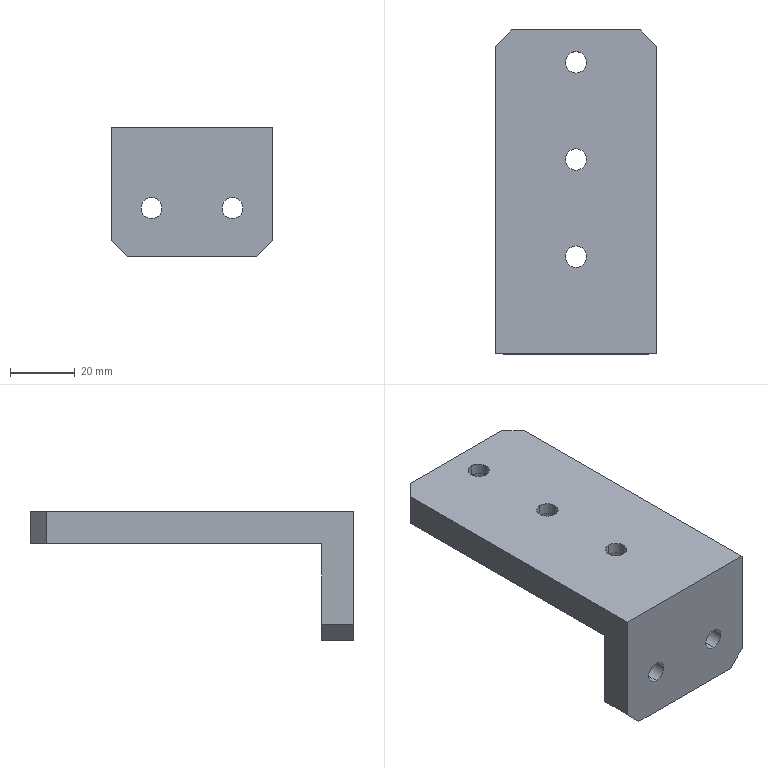Part | SolidWorks | features HoleWzd 2, Chamfer 1, ExtruThin 1 | 1 solid | 31 faces | box 50 x 100 x 40 mm | volume 61642 mm3 | cylinder 16 | plane 15 | commonest cylinder face diameters 6.6 x6 11 x6 6.5 x4
STEP:
#1=CARTESIAN_POINT('',(0.,84.5,-3.6));
#2=VERTEX_POINT('',#1);
#3=CARTESIAN_POINT('',(0.,95.5,-3.6));
#4=VERTEX_POINT('',#3);
#5=CARTESIAN_POINT('',(0.,90.,-3.6));
#6=DIRECTION('',(0.,0.,-1.));
#7=DIRECTION('',(0.,1.,0.));
#8=AXIS2_PLACEMENT_3D('',#5,#6,#7);
#9=CIRCLE('',#8,5.5);
#10=EDGE_CURVE('',#2,#4,#9,.T.);
#11=ORIENTED_EDGE('',*,*,#10,.F.);
#12=CARTESIAN_POINT('',(0.,84.5,-10.));
#13=VERTEX_POINT('',#12);
#14=CARTESIAN_POINT('',(0.,84.5,-10.));
#15=DIRECTION('',(0.,0.,-1.));
#16=VECTOR('',#15,1000.);
#17=LINE('',#14,#16);
#18=EDGE_CURVE('',#2,#13,#17,.T.);
#19=ORIENTED_EDGE('',*,*,#18,.T.);
#20=CARTESIAN_POINT('',(0.,95.5,-10.));
#21=VERTEX_POINT('',#20);
#22=CARTESIAN_POINT('',(0.,90.,-10.));
#23=DIRECTION('',(0.,0.,-1.));
#24=DIRECTION('',(0.,1.,0.));
#25=AXIS2_PLACEMENT_3D('',#22,#23,#24);
#26=CIRCLE('',#25,5.5);
#27=EDGE_CURVE('',#13,#21,#26,.T.);
#28=ORIENTED_EDGE('',*,*,#27,.T.);
#29=CARTESIAN_POINT('',(0.,95.5,-10.));
#30=DIRECTION('',(0.,0.,-1.));
#31=VECTOR('',#30,1000.);
#32=LINE('',#29,#31);
#33=EDGE_CURVE('',#4,#21,#32,.T.);
#34=ORIENTED_EDGE('',*,*,#33,.F.);
#35=EDGE_LOOP('',(#11,#19,#28,#34));
#36=FACE_OUTER_BOUND('',#35,.T.);
#37=CARTESIAN_POINT('',(0.,90.,-10.));
#38=DIRECTION('',(0.,0.,-1.));
#39=DIRECTION('',(0.,1.,0.));
#40=AXIS2_PLACEMENT_3D('',#37,#38,#39);
#41=CYLINDRICAL_SURFACE('',#40,5.5);
#42=ADVANCED_FACE('',(#36),#41,.F.);
#43=CARTESIAN_POINT('',(0.,86.7,0.));
#44=VERTEX_POINT('',#43);
#45=CARTESIAN_POINT('',(0.,93.3,0.));
#46=VERTEX_POINT('',#45);
#47=CARTESIAN_POINT('',(0.,90.,0.));
#48=DIRECTION('',(0.,0.,-1.));
#49=DIRECTION('',(0.,1.,0.));
#50=AXIS2_PLACEMENT_3D('',#47,#48,#49);
#51=CIRCLE('',#50,3.3);
#52=EDGE_CURVE('',#44,#46,#51,.T.);
#53=ORIENTED_EDGE('',*,*,#52,.F.);
#54=CARTESIAN_POINT('',(0.,86.7,-3.6));
#55=VERTEX_POINT('',#54);
#56=CARTESIAN_POINT('',(0.,86.7,-10.));
#57=DIRECTION('',(0.,0.,-1.));
#58=VECTOR('',#57,1000.);
#59=LINE('',#56,#58);
#60=EDGE_CURVE('',#44,#55,#59,.T.);
#61=ORIENTED_EDGE('',*,*,#60,.T.);
#62=CARTESIAN_POINT('',(0.,93.3,-3.6));
#63=VERTEX_POINT('',#62);
#64=CARTESIAN_POINT('',(0.,90.,-3.6));
#65=DIRECTION('',(0.,0.,-1.));
#66=DIRECTION('',(0.,1.,0.));
#67=AXIS2_PLACEMENT_3D('',#64,#65,#66);
#68=CIRCLE('',#67,3.3);
#69=EDGE_CURVE('',#55,#63,#68,.T.);
#70=ORIENTED_EDGE('',*,*,#69,.T.);
#71=CARTESIAN_POINT('',(0.,93.3,-10.));
#72=DIRECTION('',(0.,0.,-1.));
#73=VECTOR('',#72,1000.);
#74=LINE('',#71,#73);
#75=EDGE_CURVE('',#46,#63,#74,.T.);
#76=ORIENTED_EDGE('',*,*,#75,.F.);
#77=EDGE_LOOP('',(#53,#61,#70,#76));
#78=FACE_OUTER_BOUND('',#77,.T.);
#79=CARTESIAN_POINT('',(0.,90.,-10.));
#80=DIRECTION('',(0.,0.,-1.));
#81=DIRECTION('',(0.,1.,0.));
#82=AXIS2_PLACEMENT_3D('',#79,#80,#81);
#83=CYLINDRICAL_SURFACE('',#82,3.3);
#84=ADVANCED_FACE('',(#78),#83,.F.);
#85=CARTESIAN_POINT('',(0.,54.5,-3.6));
#86=VERTEX_POINT('',#85);
#87=CARTESIAN_POINT('',(0.,65.5,-3.6));
#88=VERTEX_POINT('',#87);
#89=CARTESIAN_POINT('',(0.,60.,-3.6));
#90=DIRECTION('',(0.,0.,-1.));
#91=DIRECTION('',(0.,1.,0.));
#92=AXIS2_PLACEMENT_3D('',#89,#90,#91);
#93=CIRCLE('',#92,5.5);
#94=EDGE_CURVE('',#86,#88,#93,.T.);
#95=ORIENTED_EDGE('',*,*,#94,.F.);
#96=CARTESIAN_POINT('',(0.,54.5,-10.));
#97=VERTEX_POINT('',#96);
#98=CARTESIAN_POINT('',(0.,54.5,-10.));
#99=DIRECTION('',(0.,0.,-1.));
#100=VECTOR('',#99,1000.);
#101=LINE('',#98,#100);
#102=EDGE_CURVE('',#86,#97,#101,.T.);
#103=ORIENTED_EDGE('',*,*,#102,.T.);
#104=CARTESIAN_POINT('',(0.,65.5,-10.));
#105=VERTEX_POINT('',#104);
#106=CARTESIAN_POINT('',(0.,60.,-10.));
#107=DIRECTION('',(0.,0.,-1.));
#108=DIRECTION('',(0.,1.,0.));
#109=AXIS2_PLACEMENT_3D('',#106,#107,#108);
#110=CIRCLE('',#109,5.5);
#111=EDGE_CURVE('',#97,#105,#110,.T.);
#112=ORIENTED_EDGE('',*,*,#111,.T.);
#113=CARTESIAN_POINT('',(0.,65.5,-10.));
#114=DIRECTION('',(0.,0.,-1.));
#115=VECTOR('',#114,1000.);
#116=LINE('',#113,#115);
#117=EDGE_CURVE('',#88,#105,#116,.T.);
#118=ORIENTED_EDGE('',*,*,#117,.F.);
#119=EDGE_LOOP('',(#95,#103,#112,#118));
#120=FACE_OUTER_BOUND('',#119,.T.);
#121=CARTESIAN_POINT('',(0.,60.,-10.));
#122=DIRECTION('',(0.,0.,-1.));
#123=DIRECTION('',(0.,1.,0.));
#124=AXIS2_PLACEMENT_3D('',#121,#122,#123);
#125=CYLINDRICAL_SURFACE('',#124,5.5);
#126=ADVANCED_FACE('',(#120),#125,.F.);
#127=CARTESIAN_POINT('',(0.,56.7,0.));
#128=VERTEX_POINT('',#127);
#129=CARTESIAN_POINT('',(0.,63.3,0.));
#130=VERTEX_POINT('',#129);
#131=CARTESIAN_POINT('',(0.,60.,0.));
#132=DIRECTION('',(0.,0.,-1.));
#133=DIRECTION('',(0.,1.,0.));
#134=AXIS2_PLACEMENT_3D('',#131,#132,#133);
#135=CIRCLE('',#134,3.3);
#136=EDGE_CURVE('',#128,#130,#135,.T.);
#137=ORIENTED_EDGE('',*,*,#136,.F.);
#138=CARTESIAN_POINT('',(0.,56.7,-3.6));
#139=VERTEX_POINT('',#138);
#140=CARTESIAN_POINT('',(0.,56.7,-10.));
#141=DIRECTION('',(0.,0.,-1.));
#142=VECTOR('',#141,1000.);
#143=LINE('',#140,#142);
#144=EDGE_CURVE('',#128,#139,#143,.T.);
#145=ORIENTED_EDGE('',*,*,#144,.T.);
#146=CARTESIAN_POINT('',(0.,63.3,-3.6));
#147=VERTEX_POINT('',#146);
#148=CARTESIAN_POINT('',(0.,60.,-3.6));
#149=DIRECTION('',(0.,0.,-1.));
#150=DIRECTION('',(0.,1.,0.));
#151=AXIS2_PLACEMENT_3D('',#148,#149,#150);
#152=CIRCLE('',#151,3.3);
#153=EDGE_CURVE('',#139,#147,#152,.T.);
#154=ORIENTED_EDGE('',*,*,#153,.T.);
#155=CARTESIAN_POINT('',(0.,63.3,-10.));
#156=DIRECTION('',(0.,0.,-1.));
#157=VECTOR('',#156,1000.);
#158=LINE('',#155,#157);
#159=EDGE_CURVE('',#130,#147,#158,.T.);
#160=ORIENTED_EDGE('',*,*,#159,.F.);
#161=EDGE_LOOP('',(#137,#145,#154,#160));
#162=FACE_OUTER_BOUND('',#161,.T.);
#163=CARTESIAN_POINT('',(0.,60.,-10.));
#164=DIRECTION('',(0.,0.,-1.));
#165=DIRECTION('',(0.,1.,0.));
#166=AXIS2_PLACEMENT_3D('',#163,#164,#165);
#167=CYLINDRICAL_SURFACE('',#166,3.3);
#168=ADVANCED_FACE('',(#162),#167,.F.);
#169=CARTESIAN_POINT('',(0.,24.5,-3.6));
#170=VERTEX_POINT('',#169);
#171=CARTESIAN_POINT('',(0.,35.5,-3.6));
#172=VERTEX_POINT('',#171);
#173=CARTESIAN_POINT('',(0.,30.,-3.6));
#174=DIRECTION('',(0.,0.,-1.));
#175=DIRECTION('',(0.,1.,0.));
#176=AXIS2_PLACEMENT_3D('',#173,#174,#175);
#177=CIRCLE('',#176,5.5);
#178=EDGE_CURVE('',#170,#172,#177,.T.);
#179=ORIENTED_EDGE('',*,*,#178,.F.);
#180=CARTESIAN_POINT('',(0.,24.5,-10.));
#181=VERTEX_POINT('',#180);
#182=CARTESIAN_POINT('',(0.,24.5,-10.));
#183=DIRECTION('',(0.,0.,-1.));
#184=VECTOR('',#183,1000.);
#185=LINE('',#182,#184);
#186=EDGE_CURVE('',#170,#181,#185,.T.);
#187=ORIENTED_EDGE('',*,*,#186,.T.);
#188=CARTESIAN_POINT('',(0.,35.5,-10.));
#189=VERTEX_POINT('',#188);
#190=CARTESIAN_POINT('',(0.,30.,-10.));
#191=DIRECTION('',(0.,0.,-1.));
#192=DIRECTION('',(0.,1.,0.));
#193=AXIS2_PLACEMENT_3D('',#190,#191,#192);
#194=CIRCLE('',#193,5.5);
#195=EDGE_CURVE('',#181,#189,#194,.T.);
#196=ORIENTED_EDGE('',*,*,#195,.T.);
#197=CARTESIAN_POINT('',(0.,35.5,-10.));
#198=DIRECTION('',(0.,0.,-1.));
#199=VECTOR('',#198,1000.);
#200=LINE('',#197,#199);
#201=EDGE_CURVE('',#172,#189,#200,.T.);
#202=ORIENTED_EDGE('',*,*,#201,.F.);
#203=EDGE_LOOP('',(#179,#187,#196,#202));
#204=FACE_OUTER_BOUND('',#203,.T.);
#205=CARTESIAN_POINT('',(0.,30.,-10.));
#206=DIRECTION('',(0.,0.,-1.));
#207=DIRECTION('',(0.,1.,0.));
#208=AXIS2_PLACEMENT_3D('',#205,#206,#207);
#209=CYLINDRICAL_SURFACE('',#208,5.5);
#210=ADVANCED_FACE('',(#204),#209,.F.);
#211=CARTESIAN_POINT('',(0.,26.7,0.));
#212=VERTEX_POINT('',#211);
#213=CARTESIAN_POINT('',(0.,33.3,0.));
#214=VERTEX_POINT('',#213);
#215=CARTESIAN_POINT('',(0.,30.,0.));
#216=DIRECTION('',(0.,0.,-1.));
#217=DIRECTION('',(0.,1.,0.));
#218=AXIS2_PLACEMENT_3D('',#215,#216,#217);
#219=CIRCLE('',#218,3.3);
#220=EDGE_CURVE('',#212,#214,#219,.T.);
#221=ORIENTED_EDGE('',*,*,#220,.F.);
#222=CARTESIAN_POINT('',(0.,26.7,-3.6));
#223=VERTEX_POINT('',#222);
#224=CARTESIAN_POINT('',(0.,26.7,-10.));
#225=DIRECTION('',(0.,0.,-1.));
#226=VECTOR('',#225,1000.);
#227=LINE('',#224,#226);
#228=EDGE_CURVE('',#212,#223,#227,.T.);
#229=ORIENTED_EDGE('',*,*,#228,.T.);
#230=CARTESIAN_POINT('',(0.,33.3,-3.6));
#231=VERTEX_POINT('',#230);
#232=CARTESIAN_POINT('',(0.,30.,-3.6));
#233=DIRECTION('',(0.,0.,-1.));
#234=DIRECTION('',(0.,1.,0.));
#235=AXIS2_PLACEMENT_3D('',#232,#233,#234);
#236=CIRCLE('',#235,3.3);
#237=EDGE_CURVE('',#223,#231,#236,.T.);
#238=ORIENTED_EDGE('',*,*,#237,.T.);
#239=CARTESIAN_POINT('',(0.,33.3,-10.));
#240=DIRECTION('',(0.,0.,-1.));
#241=VECTOR('',#240,1000.);
#242=LINE('',#239,#241);
#243=EDGE_CURVE('',#214,#231,#242,.T.);
#244=ORIENTED_EDGE('',*,*,#243,.F.);
#245=EDGE_LOOP('',(#221,#229,#238,#244));
#246=FACE_OUTER_BOUND('',#245,.T.);
#247=CARTESIAN_POINT('',(0.,30.,-10.));
#248=DIRECTION('',(0.,0.,-1.));
#249=DIRECTION('',(0.,1.,0.));
#250=AXIS2_PLACEMENT_3D('',#247,#248,#249);
#251=CYLINDRICAL_SURFACE('',#250,3.3);
#252=ADVANCED_FACE('',(#246),#251,.F.);
#253=CARTESIAN_POINT('',(-12.5,0.,-28.25));
#254=VERTEX_POINT('',#253);
#255=CARTESIAN_POINT('',(-12.5,0.,-21.75));
#256=VERTEX_POINT('',#255);
#257=CARTESIAN_POINT('',(-12.5,0.,-25.));
#258=DIRECTION('',(0.,1.,0.));
#259=DIRECTION('',(0.,0.,1.));
#260=AXIS2_PLACEMENT_3D('',#257,#258,#259);
#261=CIRCLE('',#260,3.25);
#262=EDGE_CURVE('',#254,#256,#261,.T.);
#263=ORIENTED_EDGE('',*,*,#262,.F.);
#264=CARTESIAN_POINT('',(-12.5,10.,-28.25));
#265=VERTEX_POINT('',#264);
#266=CARTESIAN_POINT('',(-12.5,10.,-28.25));
#267=DIRECTION('',(0.,1.,0.));
#268=VECTOR('',#267,1000.);
#269=LINE('',#266,#268);
#270=EDGE_CURVE('',#254,#265,#269,.T.);
#271=ORIENTED_EDGE('',*,*,#270,.T.);
#272=CARTESIAN_POINT('',(-12.5,10.,-21.75));
#273=VERTEX_POINT('',#272);
#274=CARTESIAN_POINT('',(-12.5,10.,-25.));
#275=DIRECTION('',(0.,1.,0.));
#276=DIRECTION('',(0.,0.,1.));
#277=AXIS2_PLACEMENT_3D('',#274,#275,#276);
#278=CIRCLE('',#277,3.25);
#279=EDGE_CURVE('',#265,#273,#278,.T.);
#280=ORIENTED_EDGE('',*,*,#279,.T.);
#281=CARTESIAN_POINT('',(-12.5,10.,-21.75));
#282=DIRECTION('',(0.,1.,0.));
#283=VECTOR('',#282,1000.);
#284=LINE('',#281,#283);
#285=EDGE_CURVE('',#256,#273,#284,.T.);
#286=ORIENTED_EDGE('',*,*,#285,.F.);
#287=EDGE_LOOP('',(#263,#271,#280,#286));
#288=FACE_OUTER_BOUND('',#287,.T.);
#289=CARTESIAN_POINT('',(-12.5,10.,-25.));
#290=DIRECTION('',(0.,1.,0.));
#291=DIRECTION('',(0.,0.,1.));
#292=AXIS2_PLACEMENT_3D('',#289,#290,#291);
#293=CYLINDRICAL_SURFACE('',#292,3.25);
#294=ADVANCED_FACE('',(#288),#293,.F.);
#295=CARTESIAN_POINT('',(12.5,0.,-28.25));
#296=VERTEX_POINT('',#295);
#297=CARTESIAN_POINT('',(12.5,0.,-21.75));
#298=VERTEX_POINT('',#297);
#299=CARTESIAN_POINT('',(12.5,0.,-25.));
#300=DIRECTION('',(0.,1.,0.));
#301=DIRECTION('',(0.,0.,1.));
#302=AXIS2_PLACEMENT_3D('',#299,#300,#301);
#303=CIRCLE('',#302,3.25);
#304=EDGE_CURVE('',#296,#298,#303,.T.);
#305=ORIENTED_EDGE('',*,*,#304,.F.);
#306=CARTESIAN_POINT('',(12.5,10.,-28.25));
#307=VERTEX_POINT('',#306);
#308=CARTESIAN_POINT('',(12.5,10.,-28.25));
#309=DIRECTION('',(0.,1.,0.));
#310=VECTOR('',#309,1000.);
#311=LINE('',#308,#310);
#312=EDGE_CURVE('',#296,#307,#311,.T.);
#313=ORIENTED_EDGE('',*,*,#312,.T.);
#314=CARTESIAN_POINT('',(12.5,10.,-21.75));
#315=VERTEX_POINT('',#314);
#316=CARTESIAN_POINT('',(12.5,10.,-25.));
#317=DIRECTION('',(0.,1.,0.));
#318=DIRECTION('',(0.,0.,1.));
#319=AXIS2_PLACEMENT_3D('',#316,#317,#318);
#320=CIRCLE('',#319,3.25);
#321=EDGE_CURVE('',#307,#315,#320,.T.);
#322=ORIENTED_EDGE('',*,*,#321,.T.);
#323=CARTESIAN_POINT('',(12.5,10.,-21.75));
#324=DIRECTION('',(0.,1.,0.));
#325=VECTOR('',#324,1000.);
#326=LINE('',#323,#325);
#327=EDGE_CURVE('',#298,#315,#326,.T.);
#328=ORIENTED_EDGE('',*,*,#327,.F.);
#329=EDGE_LOOP('',(#305,#313,#322,#328));
#330=FACE_OUTER_BOUND('',#329,.T.);
#331=CARTESIAN_POINT('',(12.5,10.,-25.));
#332=DIRECTION('',(0.,1.,0.));
#333=DIRECTION('',(0.,0.,1.));
#334=AXIS2_PLACEMENT_3D('',#331,#332,#333);
#335=CYLINDRICAL_SURFACE('',#334,3.25);
#336=ADVANCED_FACE('',(#330),#335,.F.);
#337=CARTESIAN_POINT('',(-12.5,0.,-25.));
#338=DIRECTION('',(0.,1.,0.));
#339=DIRECTION('',(0.,0.,1.));
#340=AXIS2_PLACEMENT_3D('',#337,#338,#339);
#341=CIRCLE('',#340,3.25);
#342=EDGE_CURVE('',#256,#254,#341,.T.);
#343=ORIENTED_EDGE('',*,*,#342,.T.);
#344=ORIENTED_EDGE('',*,*,#262,.T.);
#345=EDGE_LOOP('',(#343,#344));
#346=FACE_BOUND('',#345,.T.);
#347=CARTESIAN_POINT('',(12.5,0.,-25.));
#348=DIRECTION('',(0.,1.,0.));
#349=DIRECTION('',(0.,0.,1.));
#350=AXIS2_PLACEMENT_3D('',#347,#348,#349);
#351=CIRCLE('',#350,3.25);
#352=EDGE_CURVE('',#298,#296,#351,.T.);
#353=ORIENTED_EDGE('',*,*,#352,.T.);
#354=ORIENTED_EDGE('',*,*,#304,.T.);
#355=EDGE_LOOP('',(#353,#354));
#356=FACE_BOUND('',#355,.T.);
#357=CARTESIAN_POINT('',(-25.,0.,0.));
#358=VERTEX_POINT('',#357);
#359=CARTESIAN_POINT('',(-25.,0.,-35.));
#360=VERTEX_POINT('',#359);
#361=CARTESIAN_POINT('',(-25.,0.,0.));
#362=DIRECTION('',(0.,0.,-1.));
#363=VECTOR('',#362,1000.);
#364=LINE('',#361,#363);
#365=EDGE_CURVE('',#358,#360,#364,.T.);
#366=ORIENTED_EDGE('',*,*,#365,.T.);
#367=CARTESIAN_POINT('',(-20.,0.,-40.));
#368=VERTEX_POINT('',#367);
#369=CARTESIAN_POINT('',(-25.,0.,-35.));
#370=DIRECTION('',(0.7071,0.,-0.7071));
#371=VECTOR('',#370,1000.);
#372=LINE('',#369,#371);
#373=EDGE_CURVE('',#360,#368,#372,.T.);
#374=ORIENTED_EDGE('',*,*,#373,.T.);
#375=CARTESIAN_POINT('',(20.,0.,-40.));
#376=VERTEX_POINT('',#375);
#377=CARTESIAN_POINT('',(25.,0.,-40.));
#378=DIRECTION('',(-1.,0.,0.));
#379=VECTOR('',#378,1000.);
#380=LINE('',#377,#379);
#381=EDGE_CURVE('',#376,#368,#380,.T.);
#382=ORIENTED_EDGE('',*,*,#381,.F.);
#383=CARTESIAN_POINT('',(25.,0.,-35.));
#384=VERTEX_POINT('',#383);
#385=CARTESIAN_POINT('',(20.,0.,-40.));
#386=DIRECTION('',(0.7071,0.,0.7071));
#387=VECTOR('',#386,1000.);
#388=LINE('',#385,#387);
#389=EDGE_CURVE('',#376,#384,#388,.T.);
#390=ORIENTED_EDGE('',*,*,#389,.T.);
#391=CARTESIAN_POINT('',(25.,0.,0.));
#392=VERTEX_POINT('',#391);
#393=CARTESIAN_POINT('',(25.,0.,0.));
#394=DIRECTION('',(0.,0.,-1.));
#395=VECTOR('',#394,1000.);
#396=LINE('',#393,#395);
#397=EDGE_CURVE('',#392,#384,#396,.T.);
#398=ORIENTED_EDGE('',*,*,#397,.F.);
#399=CARTESIAN_POINT('',(25.,0.,0.));
#400=DIRECTION('',(-1.,0.,0.));
#401=VECTOR('',#400,1000.);
#402=LINE('',#399,#401);
#403=EDGE_CURVE('',#392,#358,#402,.T.);
#404=ORIENTED_EDGE('',*,*,#403,.T.);
#405=EDGE_LOOP('',(#366,#374,#382,#390,#398,#404));
#406=FACE_OUTER_BOUND('',#405,.T.);
#407=CARTESIAN_POINT('',(25.,0.,0.));
#408=DIRECTION('',(0.,1.,0.));
#409=DIRECTION('',(0.,0.,1.));
#410=AXIS2_PLACEMENT_3D('',#407,#408,#409);
#411=PLANE('',#410);
#412=ADVANCED_FACE('',(#346,#356,#406),#411,.F.);
#413=ORIENTED_EDGE('',*,*,#381,.T.);
#414=CARTESIAN_POINT('',(-20.,10.,-40.));
#415=VERTEX_POINT('',#414);
#416=CARTESIAN_POINT('',(-20.,10.,-40.));
#417=DIRECTION('',(0.,1.,0.));
#418=VECTOR('',#417,1000.);
#419=LINE('',#416,#418);
#420=EDGE_CURVE('',#368,#415,#419,.T.);
#421=ORIENTED_EDGE('',*,*,#420,.T.);
#422=CARTESIAN_POINT('',(20.,10.,-40.));
#423=VERTEX_POINT('',#422);
#424=CARTESIAN_POINT('',(25.,10.,-40.));
#425=DIRECTION('',(-1.,0.,0.));
#426=VECTOR('',#425,1000.);
#427=LINE('',#424,#426);
#428=EDGE_CURVE('',#423,#415,#427,.T.);
#429=ORIENTED_EDGE('',*,*,#428,.F.);
#430=CARTESIAN_POINT('',(20.,0.,-40.));
#431=DIRECTION('',(0.,-1.,0.));
#432=VECTOR('',#431,1000.);
#433=LINE('',#430,#432);
#434=EDGE_CURVE('',#423,#376,#433,.T.);
#435=ORIENTED_EDGE('',*,*,#434,.T.);
#436=EDGE_LOOP('',(#413,#421,#429,#435));
#437=FACE_OUTER_BOUND('',#436,.T.);
#438=CARTESIAN_POINT('',(25.,10.,-40.));
#439=DIRECTION('',(0.,0.,-1.));
#440=DIRECTION('',(-1.,0.,0.));
#441=AXIS2_PLACEMENT_3D('',#438,#439,#440);
#442=PLANE('',#441);
#443=ADVANCED_FACE('',(#437),#442,.T.);
#444=CARTESIAN_POINT('',(-12.5,10.,-25.));
#445=DIRECTION('',(0.,1.,0.));
#446=DIRECTION('',(0.,0.,1.));
#447=AXIS2_PLACEMENT_3D('',#444,#445,#446);
#448=CIRCLE('',#447,3.25);
#449=EDGE_CURVE('',#273,#265,#448,.T.);
#450=ORIENTED_EDGE('',*,*,#449,.F.);
#451=ORIENTED_EDGE('',*,*,#279,.F.);
#452=EDGE_LOOP('',(#450,#451));
#453=FACE_BOUND('',#452,.T.);
#454=CARTESIAN_POINT('',(12.5,10.,-25.));
#455=DIRECTION('',(0.,1.,0.));
#456=DIRECTION('',(0.,0.,1.));
#457=AXIS2_PLACEMENT_3D('',#454,#455,#456);
#458=CIRCLE('',#457,3.25);
#459=EDGE_CURVE('',#315,#307,#458,.T.);
#460=ORIENTED_EDGE('',*,*,#459,.F.);
#461=ORIENTED_EDGE('',*,*,#321,.F.);
#462=EDGE_LOOP('',(#460,#461));
#463=FACE_BOUND('',#462,.T.);
#464=ORIENTED_EDGE('',*,*,#428,.T.);
#465=CARTESIAN_POINT('',(-25.,10.,-35.));
#466=VERTEX_POINT('',#465);
#467=CARTESIAN_POINT('',(-17.5,10.,-42.5));
#468=DIRECTION('',(-0.7071,0.,0.7071));
#469=VECTOR('',#468,1000.);
#470=LINE('',#467,#469);
#471=EDGE_CURVE('',#415,#466,#470,.T.);
#472=ORIENTED_EDGE('',*,*,#471,.T.);
#473=CARTESIAN_POINT('',(-25.,10.,-10.));
#474=VERTEX_POINT('',#473);
#475=CARTESIAN_POINT('',(-25.,10.,0.));
#476=DIRECTION('',(0.,0.,-1.));
#477=VECTOR('',#476,1000.);
#478=LINE('',#475,#477);
#479=EDGE_CURVE('',#474,#466,#478,.T.);
#480=ORIENTED_EDGE('',*,*,#479,.F.);
#481=CARTESIAN_POINT('',(25.,10.,-10.));
#482=VERTEX_POINT('',#481);
#483=CARTESIAN_POINT('',(25.,10.,-10.));
#484=DIRECTION('',(-1.,0.,0.));
#485=VECTOR('',#484,1000.);
#486=LINE('',#483,#485);
#487=EDGE_CURVE('',#482,#474,#486,.T.);
#488=ORIENTED_EDGE('',*,*,#487,.F.);
#489=CARTESIAN_POINT('',(25.,10.,-35.));
#490=VERTEX_POINT('',#489);
#491=CARTESIAN_POINT('',(25.,10.,0.));
#492=DIRECTION('',(0.,0.,-1.));
#493=VECTOR('',#492,1000.);
#494=LINE('',#491,#493);
#495=EDGE_CURVE('',#482,#490,#494,.T.);
#496=ORIENTED_EDGE('',*,*,#495,.T.);
#497=CARTESIAN_POINT('',(42.5,10.,-17.5));
#498=DIRECTION('',(-0.7071,0.,-0.7071));
#499=VECTOR('',#498,1000.);
#500=LINE('',#497,#499);
#501=EDGE_CURVE('',#490,#423,#500,.T.);
#502=ORIENTED_EDGE('',*,*,#501,.T.);
#503=EDGE_LOOP('',(#464,#472,#480,#488,#496,#502));
#504=FACE_OUTER_BOUND('',#503,.T.);
#505=CARTESIAN_POINT('',(25.,10.,0.));
#506=DIRECTION('',(0.,1.,0.));
#507=DIRECTION('',(0.,0.,1.));
#508=AXIS2_PLACEMENT_3D('',#505,#506,#507);
#509=PLANE('',#508);
#510=ADVANCED_FACE('',(#453,#463,#504),#509,.T.);
#511=CARTESIAN_POINT('',(0.,90.,-10.));
#512=DIRECTION('',(0.,0.,-1.));
#513=DIRECTION('',(0.,1.,0.));
#514=AXIS2_PLACEMENT_3D('',#511,#512,#513);
#515=CIRCLE('',#514,5.5);
#516=EDGE_CURVE('',#21,#13,#515,.T.);
#517=ORIENTED_EDGE('',*,*,#516,.F.);
#518=ORIENTED_EDGE('',*,*,#27,.F.);
#519=EDGE_LOOP('',(#517,#518));
#520=FACE_BOUND('',#519,.T.);
#521=CARTESIAN_POINT('',(0.,60.,-10.));
#522=DIRECTION('',(0.,0.,-1.));
#523=DIRECTION('',(0.,1.,0.));
#524=AXIS2_PLACEMENT_3D('',#521,#522,#523);
#525=CIRCLE('',#524,5.5);
#526=EDGE_CURVE('',#105,#97,#525,.T.);
#527=ORIENTED_EDGE('',*,*,#526,.F.);
#528=ORIENTED_EDGE('',*,*,#111,.F.);
#529=EDGE_LOOP('',(#527,#528));
#530=FACE_BOUND('',#529,.T.);
#531=CARTESIAN_POINT('',(0.,30.,-10.));
#532=DIRECTION('',(0.,0.,-1.));
#533=DIRECTION('',(0.,1.,0.));
#534=AXIS2_PLACEMENT_3D('',#531,#532,#533);
#535=CIRCLE('',#534,5.5);
#536=EDGE_CURVE('',#189,#181,#535,.T.);
#537=ORIENTED_EDGE('',*,*,#536,.F.);
#538=ORIENTED_EDGE('',*,*,#195,.F.);
#539=EDGE_LOOP('',(#537,#538));
#540=FACE_BOUND('',#539,.T.);
#541=CARTESIAN_POINT('',(-25.,95.,-10.));
#542=VERTEX_POINT('',#541);
#543=CARTESIAN_POINT('',(-25.,100.,-10.));
#544=DIRECTION('',(0.,-1.,0.));
#545=VECTOR('',#544,1000.);
#546=LINE('',#543,#545);
#547=EDGE_CURVE('',#542,#474,#546,.T.);
#548=ORIENTED_EDGE('',*,*,#547,.F.);
#549=CARTESIAN_POINT('',(-20.,100.,-10.));
#550=VERTEX_POINT('',#549);
#551=CARTESIAN_POINT('',(2.5,122.5,-10.));
#552=DIRECTION('',(0.7071,0.7071,0.));
#553=VECTOR('',#552,1000.);
#554=LINE('',#551,#553);
#555=EDGE_CURVE('',#542,#550,#554,.T.);
#556=ORIENTED_EDGE('',*,*,#555,.T.);
#557=CARTESIAN_POINT('',(20.,100.,-10.));
#558=VERTEX_POINT('',#557);
#559=CARTESIAN_POINT('',(25.,100.,-10.));
#560=DIRECTION('',(-1.,0.,0.));
#561=VECTOR('',#560,1000.);
#562=LINE('',#559,#561);
#563=EDGE_CURVE('',#558,#550,#562,.T.);
#564=ORIENTED_EDGE('',*,*,#563,.F.);
#565=CARTESIAN_POINT('',(25.,95.,-10.));
#566=VERTEX_POINT('',#565);
#567=CARTESIAN_POINT('',(22.5,97.5,-10.));
#568=DIRECTION('',(0.7071,-0.7071,0.));
#569=VECTOR('',#568,1000.);
#570=LINE('',#567,#569);
#571=EDGE_CURVE('',#558,#566,#570,.T.);
#572=ORIENTED_EDGE('',*,*,#571,.T.);
#573=CARTESIAN_POINT('',(25.,100.,-10.));
#574=DIRECTION('',(0.,-1.,0.));
#575=VECTOR('',#574,1000.);
#576=LINE('',#573,#575);
#577=EDGE_CURVE('',#566,#482,#576,.T.);
#578=ORIENTED_EDGE('',*,*,#577,.T.);
#579=ORIENTED_EDGE('',*,*,#487,.T.);
#580=EDGE_LOOP('',(#548,#556,#564,#572,#578,#579));
#581=FACE_OUTER_BOUND('',#580,.T.);
#582=CARTESIAN_POINT('',(25.,100.,-10.));
#583=DIRECTION('',(0.,0.,-1.));
#584=DIRECTION('',(0.,1.,0.));
#585=AXIS2_PLACEMENT_3D('',#582,#583,#584);
#586=PLANE('',#585);
#587=ADVANCED_FACE('',(#520,#530,#540,#581),#586,.T.);
#588=ORIENTED_EDGE('',*,*,#563,.T.);
#589=CARTESIAN_POINT('',(-20.,100.,0.));
#590=VERTEX_POINT('',#589);
#591=CARTESIAN_POINT('',(-20.,100.,0.));
#592=DIRECTION('',(0.,0.,1.));
#593=VECTOR('',#592,1000.);
#594=LINE('',#591,#593);
#595=EDGE_CURVE('',#550,#590,#594,.T.);
#596=ORIENTED_EDGE('',*,*,#595,.T.);
#597=CARTESIAN_POINT('',(20.,100.,0.));
#598=VERTEX_POINT('',#597);
#599=CARTESIAN_POINT('',(25.,100.,0.));
#600=DIRECTION('',(-1.,0.,0.));
#601=VECTOR('',#600,1000.);
#602=LINE('',#599,#601);
#603=EDGE_CURVE('',#598,#590,#602,.T.);
#604=ORIENTED_EDGE('',*,*,#603,.F.);
#605=CARTESIAN_POINT('',(20.,100.,-10.));
#606=DIRECTION('',(0.,0.,-1.));
#607=VECTOR('',#606,1000.);
#608=LINE('',#605,#607);
#609=EDGE_CURVE('',#598,#558,#608,.T.);
#610=ORIENTED_EDGE('',*,*,#609,.T.);
#611=EDGE_LOOP('',(#588,#596,#604,#610));
#612=FACE_OUTER_BOUND('',#611,.T.);
#613=CARTESIAN_POINT('',(25.,100.,0.));
#614=DIRECTION('',(0.,1.,0.));
#615=DIRECTION('',(0.,0.,1.));
#616=AXIS2_PLACEMENT_3D('',#613,#614,#615);
#617=PLANE('',#616);
#618=ADVANCED_FACE('',(#612),#617,.T.);
#619=CARTESIAN_POINT('',(0.,90.,0.));
#620=DIRECTION('',(0.,0.,-1.));
#621=DIRECTION('',(0.,1.,0.));
#622=AXIS2_PLACEMENT_3D('',#619,#620,#621);
#623=CIRCLE('',#622,3.3);
#624=EDGE_CURVE('',#46,#44,#623,.T.);
#625=ORIENTED_EDGE('',*,*,#624,.T.);
#626=ORIENTED_EDGE('',*,*,#52,.T.);
#627=EDGE_LOOP('',(#625,#626));
#628=FACE_BOUND('',#627,.T.);
#629=CARTESIAN_POINT('',(0.,60.,0.));
#630=DIRECTION('',(0.,0.,-1.));
#631=DIRECTION('',(0.,1.,0.));
#632=AXIS2_PLACEMENT_3D('',#629,#630,#631);
#633=CIRCLE('',#632,3.3);
#634=EDGE_CURVE('',#130,#128,#633,.T.);
#635=ORIENTED_EDGE('',*,*,#634,.T.);
#636=ORIENTED_EDGE('',*,*,#136,.T.);
#637=EDGE_LOOP('',(#635,#636));
#638=FACE_BOUND('',#637,.T.);
#639=CARTESIAN_POINT('',(0.,30.,0.));
#640=DIRECTION('',(0.,0.,-1.));
#641=DIRECTION('',(0.,1.,0.));
#642=AXIS2_PLACEMENT_3D('',#639,#640,#641);
#643=CIRCLE('',#642,3.3);
#644=EDGE_CURVE('',#214,#212,#643,.T.);
#645=ORIENTED_EDGE('',*,*,#644,.T.);
#646=ORIENTED_EDGE('',*,*,#220,.T.);
#647=EDGE_LOOP('',(#645,#646));
#648=FACE_BOUND('',#647,.T.);
#649=ORIENTED_EDGE('',*,*,#603,.T.);
#650=CARTESIAN_POINT('',(-25.,95.,0.));
#651=VERTEX_POINT('',#650);
#652=CARTESIAN_POINT('',(-25.,95.,0.));
#653=DIRECTION('',(-0.7071,-0.7071,0.));
#654=VECTOR('',#653,1000.);
#655=LINE('',#652,#654);
#656=EDGE_CURVE('',#590,#651,#655,.T.);
#657=ORIENTED_EDGE('',*,*,#656,.T.);
#658=CARTESIAN_POINT('',(-25.,100.,0.));
#659=DIRECTION('',(0.,-1.,0.));
#660=VECTOR('',#659,1000.);
#661=LINE('',#658,#660);
#662=EDGE_CURVE('',#651,#358,#661,.T.);
#663=ORIENTED_EDGE('',*,*,#662,.T.);
#664=ORIENTED_EDGE('',*,*,#403,.F.);
#665=CARTESIAN_POINT('',(25.,95.,0.));
#666=VERTEX_POINT('',#665);
#667=CARTESIAN_POINT('',(25.,100.,0.));
#668=DIRECTION('',(0.,-1.,0.));
#669=VECTOR('',#668,1000.);
#670=LINE('',#667,#669);
#671=EDGE_CURVE('',#666,#392,#670,.T.);
#672=ORIENTED_EDGE('',*,*,#671,.F.);
#673=CARTESIAN_POINT('',(20.,100.,0.));
#674=DIRECTION('',(-0.7071,0.7071,0.));
#675=VECTOR('',#674,1000.);
#676=LINE('',#673,#675);
#677=EDGE_CURVE('',#666,#598,#676,.T.);
#678=ORIENTED_EDGE('',*,*,#677,.T.);
#679=EDGE_LOOP('',(#649,#657,#663,#664,#672,#678));
#680=FACE_OUTER_BOUND('',#679,.T.);
#681=CARTESIAN_POINT('',(25.,100.,0.));
#682=DIRECTION('',(0.,0.,-1.));
#683=DIRECTION('',(0.,1.,0.));
#684=AXIS2_PLACEMENT_3D('',#681,#682,#683);
#685=PLANE('',#684);
#686=ADVANCED_FACE('',(#628,#638,#648,#680),#685,.F.);
#687=ORIENTED_EDGE('',*,*,#397,.T.);
#688=CARTESIAN_POINT('',(25.,10.,-35.));
#689=DIRECTION('',(0.,1.,0.));
#690=VECTOR('',#689,1000.);
#691=LINE('',#688,#690);
#692=EDGE_CURVE('',#384,#490,#691,.T.);
#693=ORIENTED_EDGE('',*,*,#692,.T.);
#694=ORIENTED_EDGE('',*,*,#495,.F.);
#695=ORIENTED_EDGE('',*,*,#577,.F.);
#696=CARTESIAN_POINT('',(25.,95.,0.));
#697=DIRECTION('',(0.,0.,1.));
#698=VECTOR('',#697,1000.);
#699=LINE('',#696,#698);
#700=EDGE_CURVE('',#566,#666,#699,.T.);
#701=ORIENTED_EDGE('',*,*,#700,.T.);
#702=ORIENTED_EDGE('',*,*,#671,.T.);
#703=EDGE_LOOP('',(#687,#693,#694,#695,#701,#702));
#704=FACE_OUTER_BOUND('',#703,.T.);
#705=CARTESIAN_POINT('',(25.,0.,0.));
#706=DIRECTION('',(-1.,0.,0.));
#707=DIRECTION('',(0.,0.,1.));
#708=AXIS2_PLACEMENT_3D('',#705,#706,#707);
#709=PLANE('',#708);
#710=ADVANCED_FACE('',(#704),#709,.F.);
#711=ORIENTED_EDGE('',*,*,#479,.T.);
#712=CARTESIAN_POINT('',(-25.,0.,-35.));
#713=DIRECTION('',(0.,-1.,0.));
#714=VECTOR('',#713,1000.);
#715=LINE('',#712,#714);
#716=EDGE_CURVE('',#466,#360,#715,.T.);
#717=ORIENTED_EDGE('',*,*,#716,.T.);
#718=ORIENTED_EDGE('',*,*,#365,.F.);
#719=ORIENTED_EDGE('',*,*,#662,.F.);
#720=CARTESIAN_POINT('',(-25.,95.,0.));
#721=DIRECTION('',(0.,0.,-1.));
#722=VECTOR('',#721,1000.);
#723=LINE('',#720,#722);
#724=EDGE_CURVE('',#651,#542,#723,.T.);
#725=ORIENTED_EDGE('',*,*,#724,.T.);
#726=ORIENTED_EDGE('',*,*,#547,.T.);
#727=EDGE_LOOP('',(#711,#717,#718,#719,#725,#726));
#728=FACE_OUTER_BOUND('',#727,.T.);
#729=CARTESIAN_POINT('',(-25.,0.,0.));
#730=DIRECTION('',(-1.,0.,0.));
#731=DIRECTION('',(0.,0.,1.));
#732=AXIS2_PLACEMENT_3D('',#729,#730,#731);
#733=PLANE('',#732);
#734=ADVANCED_FACE('',(#728),#733,.T.);
#735=ORIENTED_EDGE('',*,*,#312,.F.);
#736=ORIENTED_EDGE('',*,*,#352,.F.);
#737=ORIENTED_EDGE('',*,*,#327,.T.);
#738=ORIENTED_EDGE('',*,*,#459,.T.);
#739=EDGE_LOOP('',(#735,#736,#737,#738));
#740=FACE_OUTER_BOUND('',#739,.T.);
#741=CARTESIAN_POINT('',(12.5,10.,-25.));
#742=DIRECTION('',(0.,1.,0.));
#743=DIRECTION('',(0.,0.,1.));
#744=AXIS2_PLACEMENT_3D('',#741,#742,#743);
#745=CYLINDRICAL_SURFACE('',#744,3.25);
#746=ADVANCED_FACE('',(#740),#745,.F.);
#747=ORIENTED_EDGE('',*,*,#270,.F.);
#748=ORIENTED_EDGE('',*,*,#342,.F.);
#749=ORIENTED_EDGE('',*,*,#285,.T.);
#750=ORIENTED_EDGE('',*,*,#449,.T.);
#751=EDGE_LOOP('',(#747,#748,#749,#750));
#752=FACE_OUTER_BOUND('',#751,.T.);
#753=CARTESIAN_POINT('',(-12.5,10.,-25.));
#754=DIRECTION('',(0.,1.,0.));
#755=DIRECTION('',(0.,0.,1.));
#756=AXIS2_PLACEMENT_3D('',#753,#754,#755);
#757=CYLINDRICAL_SURFACE('',#756,3.25);
#758=ADVANCED_FACE('',(#752),#757,.F.);
#759=ORIENTED_EDGE('',*,*,#228,.F.);
#760=ORIENTED_EDGE('',*,*,#644,.F.);
#761=ORIENTED_EDGE('',*,*,#243,.T.);
#762=CARTESIAN_POINT('',(0.,30.,-3.6));
#763=DIRECTION('',(0.,0.,-1.));
#764=DIRECTION('',(0.,1.,0.));
#765=AXIS2_PLACEMENT_3D('',#762,#763,#764);
#766=CIRCLE('',#765,3.3);
#767=EDGE_CURVE('',#231,#223,#766,.T.);
#768=ORIENTED_EDGE('',*,*,#767,.T.);
#769=EDGE_LOOP('',(#759,#760,#761,#768));
#770=FACE_OUTER_BOUND('',#769,.T.);
#771=CARTESIAN_POINT('',(0.,30.,-10.));
#772=DIRECTION('',(0.,0.,-1.));
#773=DIRECTION('',(0.,1.,0.));
#774=AXIS2_PLACEMENT_3D('',#771,#772,#773);
#775=CYLINDRICAL_SURFACE('',#774,3.3);
#776=ADVANCED_FACE('',(#770),#775,.F.);
#777=ORIENTED_EDGE('',*,*,#767,.F.);
#778=ORIENTED_EDGE('',*,*,#237,.F.);
#779=EDGE_LOOP('',(#777,#778));
#780=FACE_BOUND('',#779,.T.);
#781=CARTESIAN_POINT('',(0.,30.,-3.6));
#782=DIRECTION('',(0.,0.,-1.));
#783=DIRECTION('',(0.,1.,0.));
#784=AXIS2_PLACEMENT_3D('',#781,#782,#783);
#785=CIRCLE('',#784,5.5);
#786=EDGE_CURVE('',#172,#170,#785,.T.);
#787=ORIENTED_EDGE('',*,*,#786,.T.);
#788=ORIENTED_EDGE('',*,*,#178,.T.);
#789=EDGE_LOOP('',(#787,#788));
#790=FACE_OUTER_BOUND('',#789,.T.);
#791=CARTESIAN_POINT('',(3.3,30.,-3.6));
#792=DIRECTION('',(0.,0.,1.));
#793=DIRECTION('',(0.,-1.,0.));
#794=AXIS2_PLACEMENT_3D('',#791,#792,#793);
#795=PLANE('',#794);
#796=ADVANCED_FACE('',(#780,#790),#795,.F.);
#797=ORIENTED_EDGE('',*,*,#186,.F.);
#798=ORIENTED_EDGE('',*,*,#786,.F.);
#799=ORIENTED_EDGE('',*,*,#201,.T.);
#800=ORIENTED_EDGE('',*,*,#536,.T.);
#801=EDGE_LOOP('',(#797,#798,#799,#800));
#802=FACE_OUTER_BOUND('',#801,.T.);
#803=CARTESIAN_POINT('',(0.,30.,-10.));
#804=DIRECTION('',(0.,0.,-1.));
#805=DIRECTION('',(0.,1.,0.));
#806=AXIS2_PLACEMENT_3D('',#803,#804,#805);
#807=CYLINDRICAL_SURFACE('',#806,5.5);
#808=ADVANCED_FACE('',(#802),#807,.F.);
#809=ORIENTED_EDGE('',*,*,#144,.F.);
#810=ORIENTED_EDGE('',*,*,#634,.F.);
#811=ORIENTED_EDGE('',*,*,#159,.T.);
#812=CARTESIAN_POINT('',(0.,60.,-3.6));
#813=DIRECTION('',(0.,0.,-1.));
#814=DIRECTION('',(0.,1.,0.));
#815=AXIS2_PLACEMENT_3D('',#812,#813,#814);
#816=CIRCLE('',#815,3.3);
#817=EDGE_CURVE('',#147,#139,#816,.T.);
#818=ORIENTED_EDGE('',*,*,#817,.T.);
#819=EDGE_LOOP('',(#809,#810,#811,#818));
#820=FACE_OUTER_BOUND('',#819,.T.);
#821=CARTESIAN_POINT('',(0.,60.,-10.));
#822=DIRECTION('',(0.,0.,-1.));
#823=DIRECTION('',(0.,1.,0.));
#824=AXIS2_PLACEMENT_3D('',#821,#822,#823);
#825=CYLINDRICAL_SURFACE('',#824,3.3);
#826=ADVANCED_FACE('',(#820),#825,.F.);
#827=ORIENTED_EDGE('',*,*,#817,.F.);
#828=ORIENTED_EDGE('',*,*,#153,.F.);
#829=EDGE_LOOP('',(#827,#828));
#830=FACE_BOUND('',#829,.T.);
#831=CARTESIAN_POINT('',(0.,60.,-3.6));
#832=DIRECTION('',(0.,0.,-1.));
#833=DIRECTION('',(0.,1.,0.));
#834=AXIS2_PLACEMENT_3D('',#831,#832,#833);
#835=CIRCLE('',#834,5.5);
#836=EDGE_CURVE('',#88,#86,#835,.T.);
#837=ORIENTED_EDGE('',*,*,#836,.T.);
#838=ORIENTED_EDGE('',*,*,#94,.T.);
#839=EDGE_LOOP('',(#837,#838));
#840=FACE_OUTER_BOUND('',#839,.T.);
#841=CARTESIAN_POINT('',(3.3,60.,-3.6));
#842=DIRECTION('',(0.,0.,1.));
#843=DIRECTION('',(0.,-1.,0.));
#844=AXIS2_PLACEMENT_3D('',#841,#842,#843);
#845=PLANE('',#844);
#846=ADVANCED_FACE('',(#830,#840),#845,.F.);
#847=ORIENTED_EDGE('',*,*,#102,.F.);
#848=ORIENTED_EDGE('',*,*,#836,.F.);
#849=ORIENTED_EDGE('',*,*,#117,.T.);
#850=ORIENTED_EDGE('',*,*,#526,.T.);
#851=EDGE_LOOP('',(#847,#848,#849,#850));
#852=FACE_OUTER_BOUND('',#851,.T.);
#853=CARTESIAN_POINT('',(0.,60.,-10.));
#854=DIRECTION('',(0.,0.,-1.));
#855=DIRECTION('',(0.,1.,0.));
#856=AXIS2_PLACEMENT_3D('',#853,#854,#855);
#857=CYLINDRICAL_SURFACE('',#856,5.5);
#858=ADVANCED_FACE('',(#852),#857,.F.);
#859=ORIENTED_EDGE('',*,*,#60,.F.);
#860=ORIENTED_EDGE('',*,*,#624,.F.);
#861=ORIENTED_EDGE('',*,*,#75,.T.);
#862=CARTESIAN_POINT('',(0.,90.,-3.6));
#863=DIRECTION('',(0.,0.,-1.));
#864=DIRECTION('',(0.,1.,0.));
#865=AXIS2_PLACEMENT_3D('',#862,#863,#864);
#866=CIRCLE('',#865,3.3);
#867=EDGE_CURVE('',#63,#55,#866,.T.);
#868=ORIENTED_EDGE('',*,*,#867,.T.);
#869=EDGE_LOOP('',(#859,#860,#861,#868));
#870=FACE_OUTER_BOUND('',#869,.T.);
#871=CARTESIAN_POINT('',(0.,90.,-10.));
#872=DIRECTION('',(0.,0.,-1.));
#873=DIRECTION('',(0.,1.,0.));
#874=AXIS2_PLACEMENT_3D('',#871,#872,#873);
#875=CYLINDRICAL_SURFACE('',#874,3.3);
#876=ADVANCED_FACE('',(#870),#875,.F.);
#877=ORIENTED_EDGE('',*,*,#867,.F.);
#878=ORIENTED_EDGE('',*,*,#69,.F.);
#879=EDGE_LOOP('',(#877,#878));
#880=FACE_BOUND('',#879,.T.);
#881=CARTESIAN_POINT('',(0.,90.,-3.6));
#882=DIRECTION('',(0.,0.,-1.));
#883=DIRECTION('',(0.,1.,0.));
#884=AXIS2_PLACEMENT_3D('',#881,#882,#883);
#885=CIRCLE('',#884,5.5);
#886=EDGE_CURVE('',#4,#2,#885,.T.);
#887=ORIENTED_EDGE('',*,*,#886,.T.);
#888=ORIENTED_EDGE('',*,*,#10,.T.);
#889=EDGE_LOOP('',(#887,#888));
#890=FACE_OUTER_BOUND('',#889,.T.);
#891=CARTESIAN_POINT('',(3.3,90.,-3.6));
#892=DIRECTION('',(0.,0.,1.));
#893=DIRECTION('',(0.,-1.,0.));
#894=AXIS2_PLACEMENT_3D('',#891,#892,#893);
#895=PLANE('',#894);
#896=ADVANCED_FACE('',(#880,#890),#895,.F.);
#897=ORIENTED_EDGE('',*,*,#18,.F.);
#898=ORIENTED_EDGE('',*,*,#886,.F.);
#899=ORIENTED_EDGE('',*,*,#33,.T.);
#900=ORIENTED_EDGE('',*,*,#516,.T.);
#901=EDGE_LOOP('',(#897,#898,#899,#900));
#902=FACE_OUTER_BOUND('',#901,.T.);
#903=CARTESIAN_POINT('',(0.,90.,-10.));
#904=DIRECTION('',(0.,0.,-1.));
#905=DIRECTION('',(0.,1.,0.));
#906=AXIS2_PLACEMENT_3D('',#903,#904,#905);
#907=CYLINDRICAL_SURFACE('',#906,5.5);
#908=ADVANCED_FACE('',(#902),#907,.F.);
#909=ORIENTED_EDGE('',*,*,#471,.F.);
#910=ORIENTED_EDGE('',*,*,#420,.F.);
#911=ORIENTED_EDGE('',*,*,#373,.F.);
#912=ORIENTED_EDGE('',*,*,#716,.F.);
#913=EDGE_LOOP('',(#909,#910,#911,#912));
#914=FACE_OUTER_BOUND('',#913,.T.);
#915=CARTESIAN_POINT('',(-25.,0.,-35.));
#916=DIRECTION('',(0.7071,0.,0.7071));
#917=DIRECTION('',(0.,-1.,0.));
#918=AXIS2_PLACEMENT_3D('',#915,#916,#917);
#919=PLANE('',#918);
#920=ADVANCED_FACE('',(#914),#919,.F.);
#921=ORIENTED_EDGE('',*,*,#501,.F.);
#922=ORIENTED_EDGE('',*,*,#692,.F.);
#923=ORIENTED_EDGE('',*,*,#389,.F.);
#924=ORIENTED_EDGE('',*,*,#434,.F.);
#925=EDGE_LOOP('',(#921,#922,#923,#924));
#926=FACE_OUTER_BOUND('',#925,.T.);
#927=CARTESIAN_POINT('',(20.,10.,-40.));
#928=DIRECTION('',(0.7071,0.,-0.7071));
#929=DIRECTION('',(0.,1.,0.));
#930=AXIS2_PLACEMENT_3D('',#927,#928,#929);
#931=PLANE('',#930);
#932=ADVANCED_FACE('',(#926),#931,.T.);
#933=ORIENTED_EDGE('',*,*,#656,.F.);
#934=ORIENTED_EDGE('',*,*,#595,.F.);
#935=ORIENTED_EDGE('',*,*,#555,.F.);
#936=ORIENTED_EDGE('',*,*,#724,.F.);
#937=EDGE_LOOP('',(#933,#934,#935,#936));
#938=FACE_OUTER_BOUND('',#937,.T.);
#939=CARTESIAN_POINT('',(-25.,95.,0.));
#940=DIRECTION('',(0.7071,-0.7071,0.));
#941=DIRECTION('',(0.,0.,-1.));
#942=AXIS2_PLACEMENT_3D('',#939,#940,#941);
#943=PLANE('',#942);
#944=ADVANCED_FACE('',(#938),#943,.F.);
#945=ORIENTED_EDGE('',*,*,#677,.F.);
#946=ORIENTED_EDGE('',*,*,#700,.F.);
#947=ORIENTED_EDGE('',*,*,#571,.F.);
#948=ORIENTED_EDGE('',*,*,#609,.F.);
#949=EDGE_LOOP('',(#945,#946,#947,#948));
#950=FACE_OUTER_BOUND('',#949,.T.);
#951=CARTESIAN_POINT('',(20.,100.,0.));
#952=DIRECTION('',(0.7071,0.7071,0.));
#953=DIRECTION('',(0.,0.,1.));
#954=AXIS2_PLACEMENT_3D('',#951,#952,#953);
#955=PLANE('',#954);
#956=ADVANCED_FACE('',(#950),#955,.T.);
#957=CLOSED_SHELL('',(#42,#84,#126,#168,#210,#252,#294,#336,#412,#443,#510,#587,#618,#686,#710,#734,#746,#758,#776,#796,#808,#826,#846,#858,#876,#896,#908,#920,#932,#944,#956));
#958=MANIFOLD_SOLID_BREP('',#957);
#959=CARTESIAN_POINT('',(0.,0.,0.));
#960=DIRECTION('',(0.,0.,1.));
#961=DIRECTION('',(1.,0.,0.));
#962=AXIS2_PLACEMENT_3D('',#959,#960,#961);
#963=(LENGTH_UNIT()NAMED_UNIT(*)SI_UNIT(.MILLI.,.METRE.));
#964=UNCERTAINTY_MEASURE_WITH_UNIT(LENGTH_MEASURE(0.00001),#963,'','');
#965=(NAMED_UNIT(*)PLANE_ANGLE_UNIT()SI_UNIT($,.RADIAN.));
#966=(NAMED_UNIT(*)SI_UNIT($,.STERADIAN.)SOLID_ANGLE_UNIT());
#967=(GEOMETRIC_REPRESENTATION_CONTEXT(3)GLOBAL_UNCERTAINTY_ASSIGNED_CONTEXT((#964))GLOBAL_UNIT_ASSIGNED_CONTEXT((#963,#965,#966))REPRESENTATION_CONTEXT('',''));
#968=ADVANCED_BREP_SHAPE_REPRESENTATION('',(#958,#962),#967);